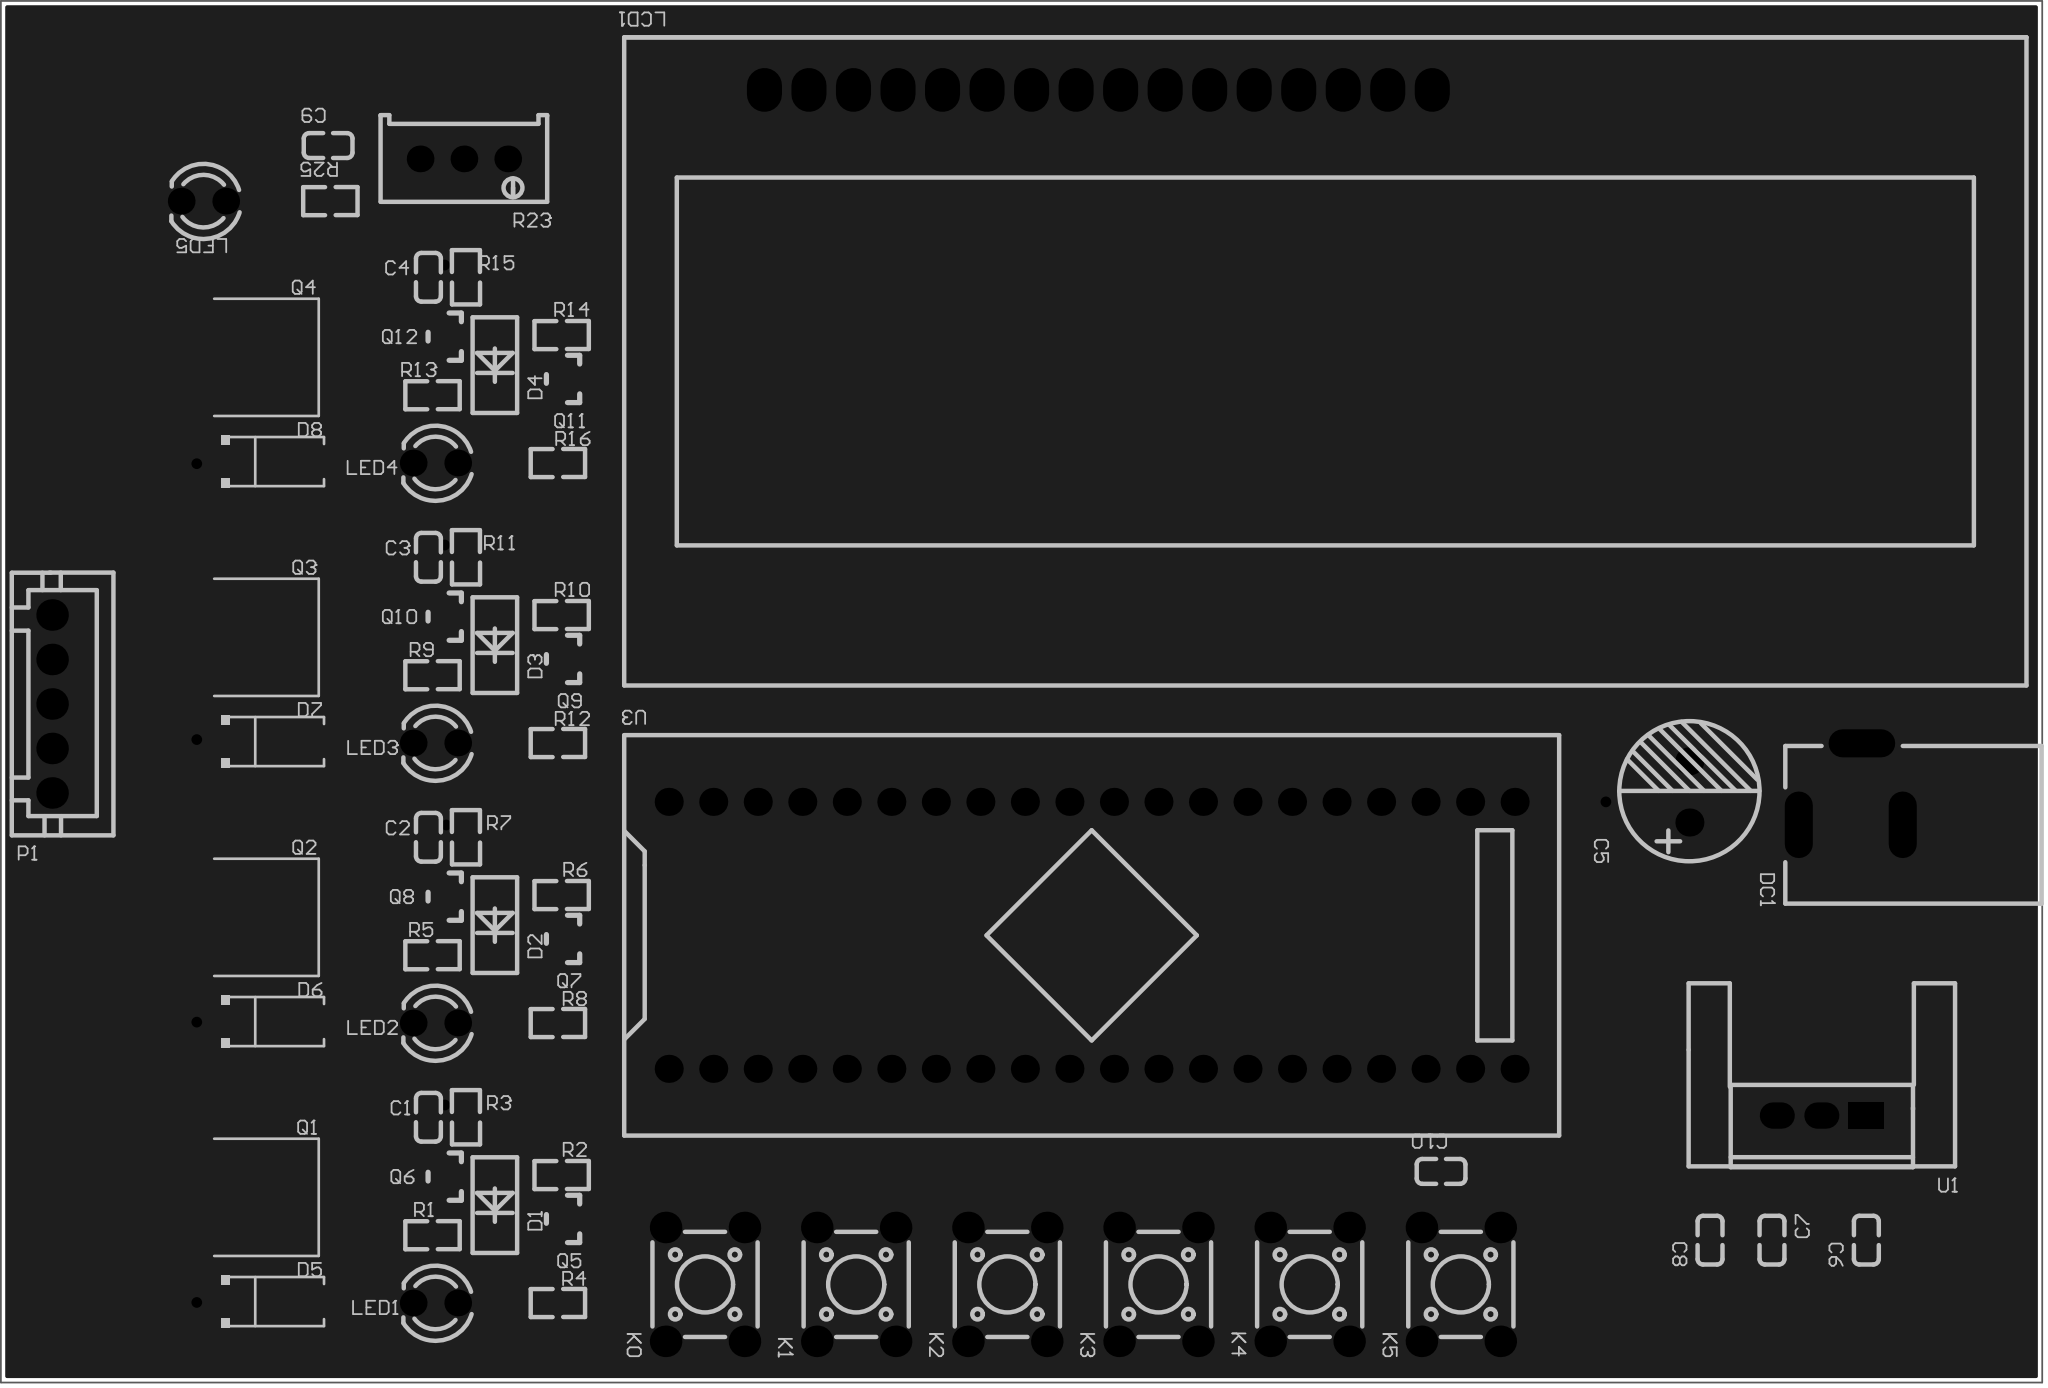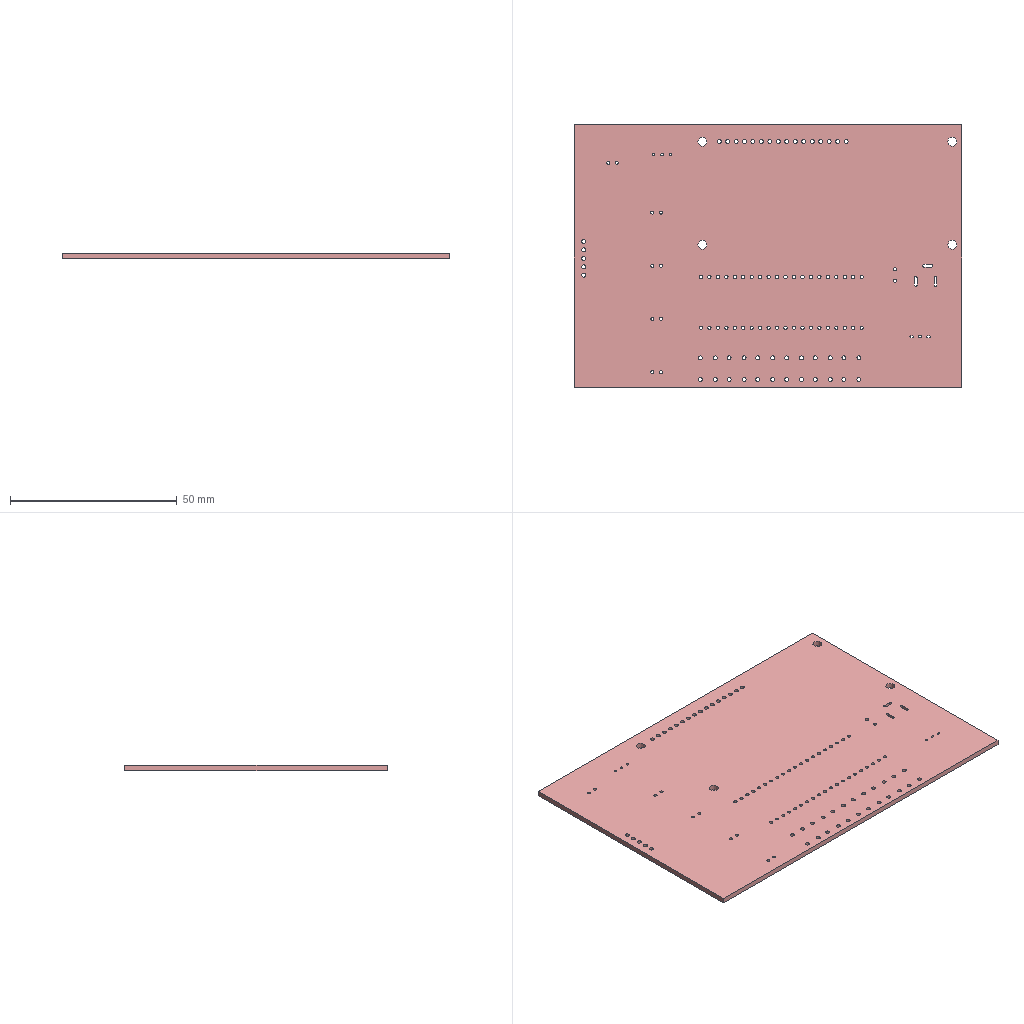Circuit board layout | Altium Designer | box 116.5 x 78.9 x 1.6 mm
Layer stack:
# Altium Designer layer stack of  (unit mm; dielectric type: 0 none, 1 core, 2 prepreg, 3 surface material)
index,name,kind,layer,copper_thickness_mm,dielectric_type,dielectric_thickness_mm,dielectric_material,dielectric_constant
0,Top Paste Mask Layer,other,,,,,,
1,Top Silkscreen Layer,other,,,,,,
2,Top Solder Mask Layer,dielectric,,,3,0.01,,3.3
3,Top Layer,copper,Top Layer,0.035,,,,
4,Dielectric1,dielectric,,,3,1.51,FR4,4.5
5,Bottom Layer,copper,Bottom Layer,0.035,,,,
6,Bottom Solder Mask Layer,dielectric,,,3,0.01,,3.3
7,Bottom Silkscreen Layer,other,,,,,,
8,Bottom Paste Mask Layer,other,,,,,,
# drill layer pairs: low layer,high layer
drill_pair,Top Layer,Bottom Layer
Part placement:
Designator,Comment,Layer,Footprint,Center-X(mm),Center-Y(mm),Rotation
C1,1nF,TopLayer,C0603,100.591,91.343,270
C2,1nF,TopLayer,C0603,100.591,107.326,270
C3,1nF,TopLayer,C0603,100.591,123.309,270
C4,1nF,TopLayer,C0603,100.591,139.292,270
C5,470uF,TopLayer,470uf,172.531,109.918,90
C6,100nF,TopLayer,C0603,182.626,84.328,90
C7,100uF,TopLayer,C0603,177.242,84.328,270
C8,100nF,TopLayer,C0603,173.708,84.328,90
C9,100nF,TopLayer,C0603,94.869,146.812,0
C10,100nF,TopLayer,C0603,158.363,88.252,0
D1,1N4148,TopLayer,1N4148,104.381,86.327,270
D2,1N4148,TopLayer,1N4148,104.381,102.31,270
D3,1N4148,TopLayer,1N4148,104.381,118.293,270
D4,1N4148,TopLayer,1N4148,104.381,134.276,270
D5,1N4007G,TopLayer,1N4007G/M7,91.908,80.823,0
D6,1N4007G,TopLayer,1N4007G/M7,91.908,96.806,0
D7,1N4007G,TopLayer,1N4007G/M7,91.908,112.789,0
D8,1N4007G,TopLayer,1N4007G/M7,91.908,128.772,0
DC1,EJ503A,TopLayer,DC-IN-TH_EJ503A,181.737,110.363,90
K0,Start/Stop,TopLayer,SW-TH_4P-L6.0-W6.0-P4.50-LS6.5,116.372,81.802,90
K1,Forward/Reverse,TopLayer,SW-TH_4P-L6.0-W6.0-P4.50-LS6.5,124.996,81.802,90
K2,Speed+10,TopLayer,SW-TH_4P-L6.0-W6.0-P4.50-LS6.5,133.62,81.802,90
K3,Speed+1,TopLayer,SW-TH_4P-L6.0-W6.0-P4.50-LS6.5,142.244,81.802,90
K4,Speed-10,TopLayer,SW-TH_4P-L6.0-W6.0-P4.50-LS6.5,150.868,81.802,90
K5,Speed-1,TopLayer,SW-TH_4P-L6.0-W6.0-P4.50-LS6.5,159.491,81.802,90
LCD1,LCM1602K-FSW-FBW-33V33,TopLayer,MODULE-TH_LCM1602K,138.811,149.987,0
P1,Motor interface,TopLayer,CONN-TH_5P-P2.54_C9900008095,79.121,114.935,90
Q1,JSM80N03D,TopLayer,TO-252-2_L6.6-W6.1-P4.57-LS9.9-BR-CW,92.951,86.772,0
Q2,JSM80N03D,TopLayer,TO-252-2_L6.6-W6.1-P4.57-LS9.9-BR-CW,92.951,102.755,0
Q3,JSM80N03D,TopLayer,TO-252-2_L6.6-W6.1-P4.57-LS9.9-BR-CW,92.951,118.738,0
Q4,JSM80N03D,TopLayer,TO-252-2_L6.6-W6.1-P4.57-LS9.9-BR-CW,92.951,134.721,0
Q5,MMS9013-H-TP,TopLayer,MMS8050-H-TP,108.122,85.54,270
Q6,MMS9013-H-TP,TopLayer,MMS8050-H-TP,101.371,87.954,270
Q7,MMS9013-H-TP,TopLayer,MMS8050-H-TP,108.122,101.523,270
Q8,MMS9013-H-TP,TopLayer,MMS8050-H-TP,101.371,103.937,270
Q9,MMS9013-H-TP,TopLayer,MMS8050-H-TP,108.122,117.506,270
Q10,MMS9013-H-TP,TopLayer,MMS8050-H-TP,101.371,119.92,270
Q11,MMS9013-H-TP,TopLayer,MMS8050-H-TP,108.122,133.489,270
Q12,MMS9013-H-TP,TopLayer,MMS8050-H-TP,101.371,135.903,270
R1,5.1Ω,TopLayer,R0603,100.825,84.613,180
R2,10kΩ,TopLayer,R0603,108.192,88.042,0
R3,1kΩ,TopLayer,R0603,102.73,91.344,270
R4,10kΩ,TopLayer,R0603,107.978,80.742,180
R5,5.1Ω,TopLayer,R0603,100.825,100.596,180
R6,10kΩ,TopLayer,R0603,108.192,104.025,0
R7,1kΩ,TopLayer,R0603,102.73,107.327,270
R8,10kΩ,TopLayer,R0603,107.978,96.725,180
R9,5.1Ω,TopLayer,R0603,100.825,116.579,180
R10,10kΩ,TopLayer,R0603,108.192,120.008,0
R11,1kΩ,TopLayer,R0603,102.73,123.31,270
R12,10kΩ,TopLayer,R0603,107.978,112.708,180
R13,5.1Ω,TopLayer,R0603,100.825,132.562,180
R14,10kΩ,TopLayer,R0603,108.192,135.991,0
R15,1kΩ,TopLayer,R0603,102.73,139.293,270
R16,10kΩ,TopLayer,R0603,107.978,128.691,180
R23,10kΩ,TopLayer,R_3296,102.616,146.05,180
R25,3kΩ,TopLayer,R0603,94.996,143.637,0
U1,LM7805,TopLayer,LM7805,180.086,91.44,180
U3,LCKFB-DKX-STM32F103C8T6,TopLayer,CONN-TH_L53.3-W22.9_STM32F103C8T6-CARD,138.43,101.727,0
LED1,3mmFIR,TopLayer,LED_TH-3mm,100.993,80.742,180
LED2,3mmFIR,TopLayer,LED_TH-3mm,100.993,96.725,180
LED3,3mmFIR,TopLayer,LED_TH-3mm,100.993,112.708,180
LED4,3mmFIR,TopLayer,LED_TH-3mm,100.993,128.691,180
LED5,3mmFIR,TopLayer,LED_TH-3mm,87.757,143.637,180
Pad and via stacks:
# Altium Designer via and pad stacks of  (unit mm). Each distinct definition once, with the count of objects using it.
# via: kind,start_layer,end_layer,hole_mm,diameter_mm,mode(0 simple;1 top-mid-bottom;2 full stack),diameter_per_layer,count,example_net
# pad: kind,layer,hole_mm,hole_type(0 round;1 square;2 slot),plating,top_size,top_shape(1 round;2 rect;3 octagon;9 rounded rect),mid_size,bottom_size,mode,footprint,size_per_layer,count,example
pad,Top Layer,0,0,plated,0.8x0.9,2,0.8x0.9,0.8x0.9,0,C0603,,18,C1.2
pad,Top Layer,0,0,plated,1.524x1.524,2,1.524x1.524,1.524x1.524,0,1N4148,,8,D1.1
pad,Top Layer,0,0,plated,1.8x1.7,2,1.8x1.7,1.8x1.7,0,1N4007G/M7,,8,D5.1
pad,Top Layer,0,0,plated,3x1.6,2,3x1.6,3x1.6,0,TO-252-2_L6.6-W6.1-P4.57-LS9.9-BR-CW,,8,Q1.1
pad,Top Layer,0,0,plated,6.2x5.8,2,6.2x5.8,6.2x5.8,0,TO-252-2_L6.6-W6.1-P4.57-LS9.9-BR-CW,,4,Q1.2
pad,Top Layer,0,0,plated,0.5x1,2,0.5x1,0.5x1,0,MMS8050-H-TP,,24,Q5.1
pad,Top Layer,0,0,plated,1x1.1,2,1x1.1,1x1.1,0,R0603,,34,R1.2
pad,Multi-Layer,1,0,plated,1.6x1.6,1,1.6x1.6,1.6x1.6,0,470uf,,2,C5.2
pad,Multi-Layer,0.8,2,plated,1.6x3.8,1,1.6x3.8,1.6x3.8,0,DC-IN-TH_EJ503A,,2,DC1.1
pad,Multi-Layer,0.8,2,plated,3.8x1.6,1,3.8x1.6,3.8x1.6,0,DC-IN-TH_EJ503A,,1,DC1.2
pad,Multi-Layer,1.2,0,plated,1.8x1.8,1,1.8x1.8,1.8x1.8,0,SW-TH_4P-L6.0-W6.0-P4.50-LS6.5,,24,K0.1
pad,Multi-Layer,1.2,0,plated,2.5x2,1,2.5x2,2.5x2,0,MODULE-TH_LCM1602K,,16,LCD1.1
pad,Multi-Layer,1.2,0,plated,1.8x1.8,1,1.8x1.8,1.8x1.8,0,CONN-TH_5P-P2.54_C9900008095,,5,P1.5
pad,Multi-Layer,0.762,0,plated,1.524x1.524,1,1.524x1.524,1.524x1.524,0,R_3296,,3,R23.2
pad,Multi-Layer,0.6,2,plated,2x1.5,2,2x1.5,2x1.5,0,LM7805,,1,U1.1
pad,Multi-Layer,0.6,2,plated,2x1.5,1,2x1.5,2x1.5,0,LM7805,,2,U1.2
pad,Multi-Layer,1,0,plated,1.6x1.6,1,1.6x1.6,1.6x1.6,0,CONN-TH_L53.3-W22.9_STM32F103C8T6-CARD,,40,U3.1
pad,Multi-Layer,0.9144,0,plated,1.524x1.524,1,1.524x1.524,1.524x1.524,0,LED_TH-3mm,,10,LED1.1
via,Top Layer,Bottom Layer,0.3048,0.61,0,,9,MT D
Copper pours:
name,layer,net,type(0 solid;1 hatched;2 none)
Top Layer-GND,Top Layer,GND,0
Bottom Layer-GND,Bottom Layer,GND,0
Design rules, without the lines most boards share:
# Altium Designer design rules of  (exported by Altium Designer, unit mm)
# columns: name | kind | enabled | priority | scope1 | scope2 | descriptor | typed fields (field=value)
creepage | 65 | enabled | 1 | All | All | Creepage Distance Constraint =(0mil) (All),(All) |